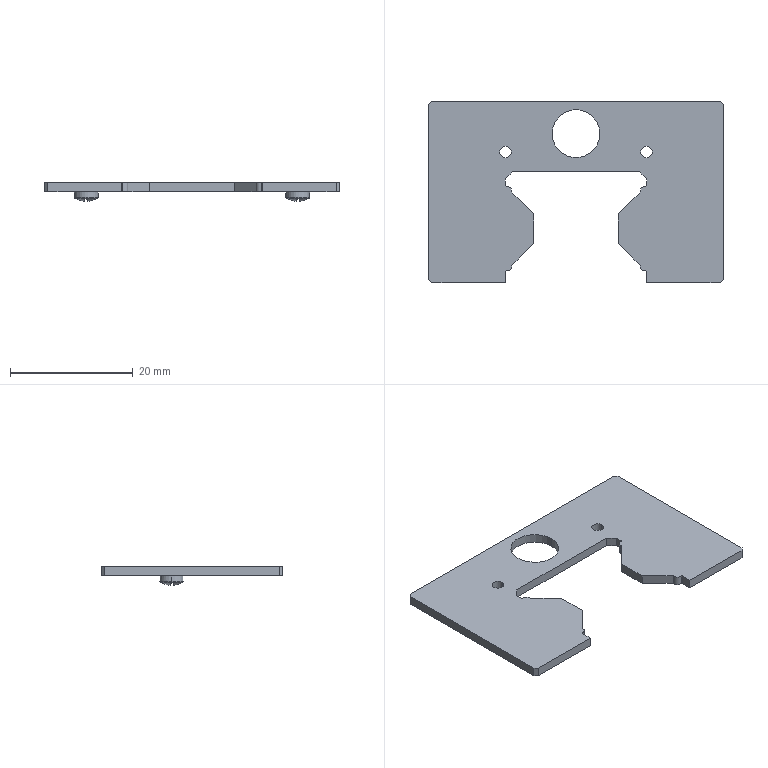Part | STEP file | 2026.6.15-Main Assembly图.sldasm-Part-24 | 1 solid | 80 faces | box 48 x 29.585 x 3.015 mm | volume 1583 mm3 | plane 54 | cylinder 18 | torus 6 | sphere 2 | commonest cylinder face diameters 1.629 x8 1.92 x4 3.84 x4 7.8 x2